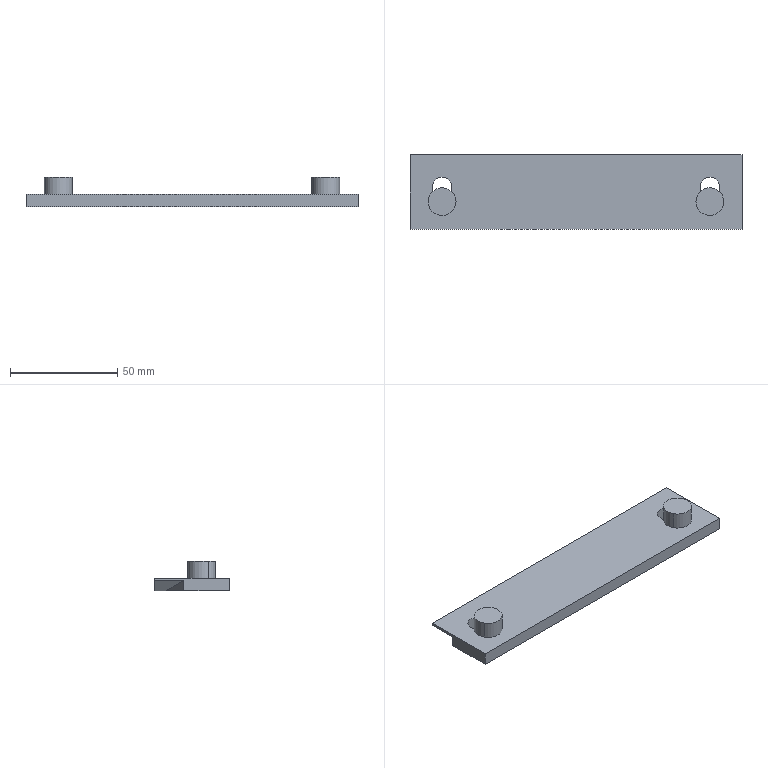Part | CATIA | 3 solids | 26 faces | box 155 x 35 x 14 mm | volume 32367 mm3 | plane 18 | cylinder 8 | commonest cylinder face diameters 9 x4 13 x4
STEP:
#1=CARTESIAN_POINT('',(-77.5,-30.,38.));
#2=VERTEX_POINT('',#1);
#3=CARTESIAN_POINT('',(-77.5,-30.,44.));
#4=VERTEX_POINT('',#3);
#5=CARTESIAN_POINT('',(-77.5,-30.,41.));
#6=DIRECTION('',(0.,0.,1.));
#7=VECTOR('',#6,1.);
#8=LINE('',#5,#7);
#9=EDGE_CURVE('',#2,#4,#8,.T.);
#10=ORIENTED_EDGE('',*,*,#9,.F.);
#11=CARTESIAN_POINT('',(77.5,-30.,38.));
#12=VERTEX_POINT('',#11);
#13=CARTESIAN_POINT('',(0.,-30.,38.));
#14=DIRECTION('',(1.,0.,0.));
#15=VECTOR('',#14,1.);
#16=LINE('',#13,#15);
#17=EDGE_CURVE('',#2,#12,#16,.T.);
#18=ORIENTED_EDGE('',*,*,#17,.T.);
#19=CARTESIAN_POINT('',(77.5,-30.,44.));
#20=VERTEX_POINT('',#19);
#21=CARTESIAN_POINT('',(77.5,-30.,41.));
#22=DIRECTION('',(0.,0.,1.));
#23=VECTOR('',#22,1.);
#24=LINE('',#21,#23);
#25=EDGE_CURVE('',#12,#20,#24,.T.);
#26=ORIENTED_EDGE('',*,*,#25,.T.);
#27=CARTESIAN_POINT('',(0.,-30.,44.));
#28=DIRECTION('',(1.,0.,0.));
#29=VECTOR('',#28,1.);
#30=LINE('',#27,#29);
#31=EDGE_CURVE('',#4,#20,#30,.T.);
#32=ORIENTED_EDGE('',*,*,#31,.F.);
#33=EDGE_LOOP('',(#10,#18,#26,#32));
#34=FACE_OUTER_BOUND('',#33,.T.);
#35=CARTESIAN_POINT('',(-77.5,-30.,38.));
#36=DIRECTION('',(0.,-1.,0.));
#37=DIRECTION('',(1.,0.,0.));
#38=AXIS2_PLACEMENT_3D('',#35,#36,#37);
#39=PLANE('',#38);
#40=ADVANCED_FACE('',(#34),#39,.T.);
#41=CARTESIAN_POINT('',(77.5,-8.66,42.874));
#42=VERTEX_POINT('',#41);
#43=CARTESIAN_POINT('',(77.5,-8.66,38.));
#44=VERTEX_POINT('',#43);
#45=CARTESIAN_POINT('',(77.5,-8.66,40.437));
#46=DIRECTION('',(0.,0.,-1.));
#47=VECTOR('',#46,1.);
#48=LINE('',#45,#47);
#49=EDGE_CURVE('',#42,#44,#48,.T.);
#50=ORIENTED_EDGE('',*,*,#49,.F.);
#51=CARTESIAN_POINT('',(77.5,5.,42.874));
#52=VERTEX_POINT('',#51);
#53=CARTESIAN_POINT('',(77.5,-1.83,42.874));
#54=DIRECTION('',(0.,1.,0.));
#55=VECTOR('',#54,1.);
#56=LINE('',#53,#55);
#57=EDGE_CURVE('',#42,#52,#56,.T.);
#58=ORIENTED_EDGE('',*,*,#57,.T.);
#59=CARTESIAN_POINT('',(77.5,5.,44.));
#60=VERTEX_POINT('',#59);
#61=CARTESIAN_POINT('',(77.5,5.,43.437));
#62=DIRECTION('',(0.,0.,1.));
#63=VECTOR('',#62,1.);
#64=LINE('',#61,#63);
#65=EDGE_CURVE('',#52,#60,#64,.T.);
#66=ORIENTED_EDGE('',*,*,#65,.T.);
#67=CARTESIAN_POINT('',(77.5,-12.5,44.));
#68=DIRECTION('',(0.,-1.,0.));
#69=VECTOR('',#68,1.);
#70=LINE('',#67,#69);
#71=EDGE_CURVE('',#20,#60,#70,.F.);
#72=ORIENTED_EDGE('',*,*,#71,.F.);
#73=ORIENTED_EDGE('',*,*,#25,.F.);
#74=CARTESIAN_POINT('',(77.5,-19.33,38.));
#75=DIRECTION('',(0.,-1.,0.));
#76=VECTOR('',#75,1.);
#77=LINE('',#74,#76);
#78=EDGE_CURVE('',#12,#44,#77,.F.);
#79=ORIENTED_EDGE('',*,*,#78,.T.);
#80=EDGE_LOOP('',(#50,#58,#66,#72,#73,#79));
#81=FACE_OUTER_BOUND('',#80,.T.);
#82=CARTESIAN_POINT('',(77.5,5.,38.));
#83=DIRECTION('',(-1.,0.,0.));
#84=DIRECTION('',(0.,-1.,0.));
#85=AXIS2_PLACEMENT_3D('',#82,#83,#84);
#86=PLANE('',#85);
#87=ADVANCED_FACE('',(#81),#86,.F.);
#88=CARTESIAN_POINT('',(-77.5,-8.66,42.874));
#89=VERTEX_POINT('',#88);
#90=CARTESIAN_POINT('',(-77.5,5.,42.874));
#91=VERTEX_POINT('',#90);
#92=CARTESIAN_POINT('',(-77.5,-1.83,42.874));
#93=DIRECTION('',(0.,1.,0.));
#94=VECTOR('',#93,1.);
#95=LINE('',#92,#94);
#96=EDGE_CURVE('',#89,#91,#95,.T.);
#97=ORIENTED_EDGE('',*,*,#96,.F.);
#98=CARTESIAN_POINT('',(-77.5,-8.66,38.));
#99=VERTEX_POINT('',#98);
#100=CARTESIAN_POINT('',(-77.5,-8.66,40.437));
#101=DIRECTION('',(0.,0.,-1.));
#102=VECTOR('',#101,1.);
#103=LINE('',#100,#102);
#104=EDGE_CURVE('',#89,#99,#103,.T.);
#105=ORIENTED_EDGE('',*,*,#104,.T.);
#106=CARTESIAN_POINT('',(-77.5,-19.33,38.));
#107=DIRECTION('',(0.,1.,0.));
#108=VECTOR('',#107,1.);
#109=LINE('',#106,#108);
#110=EDGE_CURVE('',#99,#2,#109,.F.);
#111=ORIENTED_EDGE('',*,*,#110,.T.);
#112=ORIENTED_EDGE('',*,*,#9,.T.);
#113=CARTESIAN_POINT('',(-77.5,5.,44.));
#114=VERTEX_POINT('',#113);
#115=CARTESIAN_POINT('',(-77.5,-12.5,44.));
#116=DIRECTION('',(0.,1.,0.));
#117=VECTOR('',#116,1.);
#118=LINE('',#115,#117);
#119=EDGE_CURVE('',#114,#4,#118,.F.);
#120=ORIENTED_EDGE('',*,*,#119,.F.);
#121=CARTESIAN_POINT('',(-77.5,5.,43.437));
#122=DIRECTION('',(0.,0.,1.));
#123=VECTOR('',#122,1.);
#124=LINE('',#121,#123);
#125=EDGE_CURVE('',#91,#114,#124,.T.);
#126=ORIENTED_EDGE('',*,*,#125,.F.);
#127=EDGE_LOOP('',(#97,#105,#111,#112,#120,#126));
#128=FACE_OUTER_BOUND('',#127,.T.);
#129=CARTESIAN_POINT('',(-77.5,-30.,38.));
#130=DIRECTION('',(1.,0.,0.));
#131=DIRECTION('',(0.,1.,0.));
#132=AXIS2_PLACEMENT_3D('',#129,#130,#131);
#133=PLANE('',#132);
#134=ADVANCED_FACE('',(#128),#133,.F.);
#135=CARTESIAN_POINT('',(62.5,5.,38.));
#136=VERTEX_POINT('',#135);
#137=CARTESIAN_POINT('',(-62.5,5.,38.));
#138=VERTEX_POINT('',#137);
#139=CARTESIAN_POINT('',(0.,5.,38.));
#140=DIRECTION('',(-1.,0.,0.));
#141=VECTOR('',#140,1.);
#142=LINE('',#139,#141);
#143=EDGE_CURVE('',#136,#138,#142,.T.);
#144=ORIENTED_EDGE('',*,*,#143,.T.);
#145=CARTESIAN_POINT('',(-70.,5.,40.437));
#146=DIRECTION('',(-0.9511,0.,0.309));
#147=VECTOR('',#146,1.);
#148=LINE('',#145,#147);
#149=EDGE_CURVE('',#138,#91,#148,.T.);
#150=ORIENTED_EDGE('',*,*,#149,.T.);
#151=ORIENTED_EDGE('',*,*,#125,.T.);
#152=CARTESIAN_POINT('',(0.,5.,44.));
#153=DIRECTION('',(-1.,0.,0.));
#154=VECTOR('',#153,1.);
#155=LINE('',#152,#154);
#156=EDGE_CURVE('',#60,#114,#155,.T.);
#157=ORIENTED_EDGE('',*,*,#156,.F.);
#158=ORIENTED_EDGE('',*,*,#65,.F.);
#159=CARTESIAN_POINT('',(70.,5.,40.437));
#160=DIRECTION('',(0.9511,0.,0.309));
#161=VECTOR('',#160,1.);
#162=LINE('',#159,#161);
#163=EDGE_CURVE('',#136,#52,#162,.T.);
#164=ORIENTED_EDGE('',*,*,#163,.F.);
#165=EDGE_LOOP('',(#144,#150,#151,#157,#158,#164));
#166=FACE_OUTER_BOUND('',#165,.T.);
#167=CARTESIAN_POINT('',(77.5,5.,38.));
#168=DIRECTION('',(0.,1.,0.));
#169=DIRECTION('',(-1.,0.,0.));
#170=AXIS2_PLACEMENT_3D('',#167,#168,#169);
#171=PLANE('',#170);
#172=ADVANCED_FACE('',(#166),#171,.T.);
#173=CARTESIAN_POINT('',(62.5,0.,38.));
#174=VERTEX_POINT('',#173);
#175=CARTESIAN_POINT('',(77.5,-8.66,42.874));
#176=CARTESIAN_POINT('',(62.5,0.,38.));
#177=B_SPLINE_CURVE_WITH_KNOTS('',1,(#175,#176),.UNSPECIFIED.,.F.,.U.,(2,2),(-2.999,14.994),.UNSPECIFIED.);
#178=EDGE_CURVE('',#174,#42,#177,.F.);
#179=ORIENTED_EDGE('',*,*,#178,.T.);
#180=ORIENTED_EDGE('',*,*,#49,.T.);
#181=CARTESIAN_POINT('',(75.,-7.217,38.));
#182=DIRECTION('',(0.866,-0.5,0.));
#183=VECTOR('',#182,1.);
#184=LINE('',#181,#183);
#185=EDGE_CURVE('',#174,#44,#184,.T.);
#186=ORIENTED_EDGE('',*,*,#185,.F.);
#187=EDGE_LOOP('',(#179,#180,#186));
#188=FACE_OUTER_BOUND('',#187,.T.);
#189=CARTESIAN_POINT('',(62.5,0.,38.));
#190=DIRECTION('',(0.5,0.866,0.));
#191=DIRECTION('',(0.,0.,1.));
#192=AXIS2_PLACEMENT_3D('',#189,#190,#191);
#193=PLANE('',#192);
#194=ADVANCED_FACE('',(#188),#193,.T.);
#195=ORIENTED_EDGE('',*,*,#163,.T.);
#196=ORIENTED_EDGE('',*,*,#57,.F.);
#197=ORIENTED_EDGE('',*,*,#178,.F.);
#198=CARTESIAN_POINT('',(62.5,5.,38.));
#199=DIRECTION('',(0.,-1.,0.));
#200=VECTOR('',#199,1.);
#201=LINE('',#198,#200);
#202=EDGE_CURVE('',#174,#136,#201,.F.);
#203=ORIENTED_EDGE('',*,*,#202,.T.);
#204=EDGE_LOOP('',(#195,#196,#197,#203));
#205=FACE_OUTER_BOUND('',#204,.T.);
#206=CARTESIAN_POINT('',(62.5,10.,38.));
#207=DIRECTION('',(-0.309,0.,0.9511));
#208=DIRECTION('',(0.,-1.,0.));
#209=AXIS2_PLACEMENT_3D('',#206,#207,#208);
#210=PLANE('',#209);
#211=ADVANCED_FACE('',(#205),#210,.F.);
#212=CARTESIAN_POINT('',(-62.5,0.,38.));
#213=VERTEX_POINT('',#212);
#214=CARTESIAN_POINT('',(-75.,-7.217,38.));
#215=DIRECTION('',(-0.866,-0.5,0.));
#216=VECTOR('',#215,1.);
#217=LINE('',#214,#216);
#218=EDGE_CURVE('',#213,#99,#217,.T.);
#219=ORIENTED_EDGE('',*,*,#218,.T.);
#220=ORIENTED_EDGE('',*,*,#104,.F.);
#221=CARTESIAN_POINT('',(-77.5,-8.66,42.874));
#222=CARTESIAN_POINT('',(-62.5,0.,38.));
#223=B_SPLINE_CURVE_WITH_KNOTS('',1,(#221,#222),.UNSPECIFIED.,.F.,.U.,(2,2),(-2.999,14.994),.UNSPECIFIED.);
#224=EDGE_CURVE('',#213,#89,#223,.F.);
#225=ORIENTED_EDGE('',*,*,#224,.F.);
#226=EDGE_LOOP('',(#219,#220,#225));
#227=FACE_OUTER_BOUND('',#226,.T.);
#228=CARTESIAN_POINT('',(-62.5,0.,38.));
#229=DIRECTION('',(0.5,-0.866,0.));
#230=DIRECTION('',(0.,0.,1.));
#231=AXIS2_PLACEMENT_3D('',#228,#229,#230);
#232=PLANE('',#231);
#233=ADVANCED_FACE('',(#227),#232,.F.);
#234=CARTESIAN_POINT('',(-62.5,5.,38.));
#235=DIRECTION('',(0.,-1.,0.));
#236=VECTOR('',#235,1.);
#237=LINE('',#234,#236);
#238=EDGE_CURVE('',#213,#138,#237,.F.);
#239=ORIENTED_EDGE('',*,*,#238,.F.);
#240=ORIENTED_EDGE('',*,*,#224,.T.);
#241=ORIENTED_EDGE('',*,*,#96,.T.);
#242=ORIENTED_EDGE('',*,*,#149,.F.);
#243=EDGE_LOOP('',(#239,#240,#241,#242));
#244=FACE_OUTER_BOUND('',#243,.T.);
#245=CARTESIAN_POINT('',(-62.5,10.,38.));
#246=DIRECTION('',(-0.309,0.,-0.9511));
#247=DIRECTION('',(0.,-1.,0.));
#248=AXIS2_PLACEMENT_3D('',#245,#246,#247);
#249=PLANE('',#248);
#250=ADVANCED_FACE('',(#244),#249,.T.);
#251=ORIENTED_EDGE('',*,*,#143,.F.);
#252=ORIENTED_EDGE('',*,*,#202,.F.);
#253=ORIENTED_EDGE('',*,*,#185,.T.);
#254=ORIENTED_EDGE('',*,*,#78,.F.);
#255=ORIENTED_EDGE('',*,*,#17,.F.);
#256=ORIENTED_EDGE('',*,*,#110,.F.);
#257=ORIENTED_EDGE('',*,*,#218,.F.);
#258=ORIENTED_EDGE('',*,*,#238,.T.);
#259=EDGE_LOOP('',(#251,#252,#253,#254,#255,#256,#257,#258));
#260=FACE_OUTER_BOUND('',#259,.T.);
#261=CARTESIAN_POINT('',(-58.,-10.,38.));
#262=VERTEX_POINT('',#261);
#263=CARTESIAN_POINT('',(-58.,-17.,38.));
#264=VERTEX_POINT('',#263);
#265=CARTESIAN_POINT('',(-58.,-13.5,38.));
#266=DIRECTION('',(0.,-1.,0.));
#267=VECTOR('',#266,1.);
#268=LINE('',#265,#267);
#269=EDGE_CURVE('',#262,#264,#268,.T.);
#270=ORIENTED_EDGE('',*,*,#269,.F.);
#271=CARTESIAN_POINT('',(-67.,-10.,38.));
#272=VERTEX_POINT('',#271);
#273=CARTESIAN_POINT('',(-62.5,-10.,38.));
#274=DIRECTION('',(0.,0.,1.));
#275=AXIS2_PLACEMENT_3D('',#273,#274,$);
#276=CIRCLE('',#275,4.5);
#277=EDGE_CURVE('',#262,#272,#276,.T.);
#278=ORIENTED_EDGE('',*,*,#277,.T.);
#279=CARTESIAN_POINT('',(-67.,-17.,38.));
#280=VERTEX_POINT('',#279);
#281=CARTESIAN_POINT('',(-67.,-13.5,38.));
#282=DIRECTION('',(0.,-1.,0.));
#283=VECTOR('',#282,1.);
#284=LINE('',#281,#283);
#285=EDGE_CURVE('',#272,#280,#284,.T.);
#286=ORIENTED_EDGE('',*,*,#285,.T.);
#287=CARTESIAN_POINT('',(-62.5,-17.,38.));
#288=DIRECTION('',(0.,0.,1.));
#289=AXIS2_PLACEMENT_3D('',#287,#288,$);
#290=CIRCLE('',#289,4.5);
#291=EDGE_CURVE('',#280,#264,#290,.T.);
#292=ORIENTED_EDGE('',*,*,#291,.T.);
#293=EDGE_LOOP('',(#270,#278,#286,#292));
#294=FACE_BOUND('',#293,.T.);
#295=CARTESIAN_POINT('',(67.,-10.,38.));
#296=VERTEX_POINT('',#295);
#297=CARTESIAN_POINT('',(58.,-10.,38.));
#298=VERTEX_POINT('',#297);
#299=CARTESIAN_POINT('',(62.5,-10.,38.));
#300=DIRECTION('',(0.,0.,1.));
#301=AXIS2_PLACEMENT_3D('',#299,#300,$);
#302=CIRCLE('',#301,4.5);
#303=EDGE_CURVE('',#296,#298,#302,.T.);
#304=ORIENTED_EDGE('',*,*,#303,.T.);
#305=CARTESIAN_POINT('',(58.,-17.,38.));
#306=VERTEX_POINT('',#305);
#307=CARTESIAN_POINT('',(58.,-13.5,38.));
#308=DIRECTION('',(0.,-1.,0.));
#309=VECTOR('',#308,1.);
#310=LINE('',#307,#309);
#311=EDGE_CURVE('',#298,#306,#310,.T.);
#312=ORIENTED_EDGE('',*,*,#311,.T.);
#313=CARTESIAN_POINT('',(67.,-17.,38.));
#314=VERTEX_POINT('',#313);
#315=CARTESIAN_POINT('',(62.5,-17.,38.));
#316=DIRECTION('',(0.,0.,1.));
#317=AXIS2_PLACEMENT_3D('',#315,#316,$);
#318=CIRCLE('',#317,4.5);
#319=EDGE_CURVE('',#306,#314,#318,.T.);
#320=ORIENTED_EDGE('',*,*,#319,.T.);
#321=CARTESIAN_POINT('',(67.,-13.5,38.));
#322=DIRECTION('',(0.,-1.,0.));
#323=VECTOR('',#322,1.);
#324=LINE('',#321,#323);
#325=EDGE_CURVE('',#296,#314,#324,.T.);
#326=ORIENTED_EDGE('',*,*,#325,.F.);
#327=EDGE_LOOP('',(#304,#312,#320,#326));
#328=FACE_BOUND('',#327,.T.);
#329=CARTESIAN_POINT('',(0.,0.,38.));
#330=DIRECTION('',(0.,0.,1.));
#331=DIRECTION('',(1.,0.,0.));
#332=AXIS2_PLACEMENT_3D('',#329,#330,#331);
#333=PLANE('',#332);
#334=ADVANCED_FACE('',(#260,#294,#328),#333,.F.);
#335=ORIENTED_EDGE('',*,*,#156,.T.);
#336=ORIENTED_EDGE('',*,*,#119,.T.);
#337=ORIENTED_EDGE('',*,*,#31,.T.);
#338=ORIENTED_EDGE('',*,*,#71,.T.);
#339=EDGE_LOOP('',(#335,#336,#337,#338));
#340=FACE_OUTER_BOUND('',#339,.T.);
#341=CARTESIAN_POINT('',(-58.,-17.,44.));
#342=VERTEX_POINT('',#341);
#343=CARTESIAN_POINT('',(-58.,-10.,44.));
#344=VERTEX_POINT('',#343);
#345=CARTESIAN_POINT('',(-58.,-13.5,44.));
#346=DIRECTION('',(0.,-1.,0.));
#347=VECTOR('',#346,1.);
#348=LINE('',#345,#347);
#349=EDGE_CURVE('',#342,#344,#348,.F.);
#350=ORIENTED_EDGE('',*,*,#349,.F.);
#351=CARTESIAN_POINT('',(-67.,-17.,44.));
#352=VERTEX_POINT('',#351);
#353=CARTESIAN_POINT('',(-62.5,-17.,44.));
#354=DIRECTION('',(0.,0.,1.));
#355=AXIS2_PLACEMENT_3D('',#353,#354,$);
#356=CIRCLE('',#355,4.5);
#357=EDGE_CURVE('',#352,#342,#356,.T.);
#358=ORIENTED_EDGE('',*,*,#357,.F.);
#359=CARTESIAN_POINT('',(-67.,-10.,44.));
#360=VERTEX_POINT('',#359);
#361=CARTESIAN_POINT('',(-67.,-13.5,44.));
#362=DIRECTION('',(0.,-1.,0.));
#363=VECTOR('',#362,1.);
#364=LINE('',#361,#363);
#365=EDGE_CURVE('',#360,#352,#364,.T.);
#366=ORIENTED_EDGE('',*,*,#365,.F.);
#367=CARTESIAN_POINT('',(-62.5,-10.,44.));
#368=DIRECTION('',(0.,0.,1.));
#369=AXIS2_PLACEMENT_3D('',#367,#368,$);
#370=CIRCLE('',#369,4.5);
#371=EDGE_CURVE('',#344,#360,#370,.T.);
#372=ORIENTED_EDGE('',*,*,#371,.F.);
#373=EDGE_LOOP('',(#350,#358,#366,#372));
#374=FACE_BOUND('',#373,.T.);
#375=CARTESIAN_POINT('',(67.,-10.,44.));
#376=VERTEX_POINT('',#375);
#377=CARTESIAN_POINT('',(58.,-10.,44.));
#378=VERTEX_POINT('',#377);
#379=CARTESIAN_POINT('',(62.5,-10.,44.));
#380=DIRECTION('',(0.,0.,1.));
#381=AXIS2_PLACEMENT_3D('',#379,#380,$);
#382=CIRCLE('',#381,4.5);
#383=EDGE_CURVE('',#376,#378,#382,.T.);
#384=ORIENTED_EDGE('',*,*,#383,.F.);
#385=CARTESIAN_POINT('',(67.,-17.,44.));
#386=VERTEX_POINT('',#385);
#387=CARTESIAN_POINT('',(67.,-13.5,44.));
#388=DIRECTION('',(0.,-1.,0.));
#389=VECTOR('',#388,1.);
#390=LINE('',#387,#389);
#391=EDGE_CURVE('',#386,#376,#390,.F.);
#392=ORIENTED_EDGE('',*,*,#391,.F.);
#393=CARTESIAN_POINT('',(58.,-17.,44.));
#394=VERTEX_POINT('',#393);
#395=CARTESIAN_POINT('',(62.5,-17.,44.));
#396=DIRECTION('',(0.,0.,1.));
#397=AXIS2_PLACEMENT_3D('',#395,#396,$);
#398=CIRCLE('',#397,4.5);
#399=EDGE_CURVE('',#394,#386,#398,.T.);
#400=ORIENTED_EDGE('',*,*,#399,.F.);
#401=CARTESIAN_POINT('',(58.,-13.5,44.));
#402=DIRECTION('',(0.,-1.,0.));
#403=VECTOR('',#402,1.);
#404=LINE('',#401,#403);
#405=EDGE_CURVE('',#378,#394,#404,.T.);
#406=ORIENTED_EDGE('',*,*,#405,.F.);
#407=EDGE_LOOP('',(#384,#392,#400,#406));
#408=FACE_BOUND('',#407,.T.);
#409=CARTESIAN_POINT('',(0.,0.,44.));
#410=DIRECTION('',(0.,0.,1.));
#411=DIRECTION('',(1.,0.,0.));
#412=AXIS2_PLACEMENT_3D('',#409,#410,#411);
#413=PLANE('',#412);
#414=ADVANCED_FACE('',(#340,#374,#408),#413,.T.);
#415=ORIENTED_EDGE('',*,*,#303,.F.);
#416=CARTESIAN_POINT('',(67.,-10.,34.));
#417=DIRECTION('',(0.,0.,1.));
#418=VECTOR('',#417,1.);
#419=LINE('',#416,#418);
#420=EDGE_CURVE('',#376,#296,#419,.F.);
#421=ORIENTED_EDGE('',*,*,#420,.F.);
#422=ORIENTED_EDGE('',*,*,#383,.T.);
#423=CARTESIAN_POINT('',(58.,-10.,34.));
#424=DIRECTION('',(0.,0.,1.));
#425=VECTOR('',#424,1.);
#426=LINE('',#423,#425);
#427=EDGE_CURVE('',#378,#298,#426,.F.);
#428=ORIENTED_EDGE('',*,*,#427,.T.);
#429=EDGE_LOOP('',(#415,#421,#422,#428));
#430=FACE_OUTER_BOUND('',#429,.T.);
#431=CARTESIAN_POINT('',(62.5,-10.,34.));
#432=DIRECTION('',(0.,0.,1.));
#433=DIRECTION('',(1.,0.,0.));
#434=AXIS2_PLACEMENT_3D('',#431,#432,#433);
#435=CYLINDRICAL_SURFACE('',#434,4.5);
#436=ADVANCED_FACE('',(#430),#435,.F.);
#437=ORIENTED_EDGE('',*,*,#427,.F.);
#438=ORIENTED_EDGE('',*,*,#405,.T.);
#439=CARTESIAN_POINT('',(58.,-17.,41.));
#440=DIRECTION('',(0.,0.,-1.));
#441=VECTOR('',#440,1.);
#442=LINE('',#439,#441);
#443=EDGE_CURVE('',#394,#306,#442,.T.);
#444=ORIENTED_EDGE('',*,*,#443,.T.);
#445=ORIENTED_EDGE('',*,*,#311,.F.);
#446=EDGE_LOOP('',(#437,#438,#444,#445));
#447=FACE_OUTER_BOUND('',#446,.T.);
#448=CARTESIAN_POINT('',(58.,-10.,44.));
#449=DIRECTION('',(1.,0.,0.));
#450=DIRECTION('',(0.,-1.,0.));
#451=AXIS2_PLACEMENT_3D('',#448,#449,#450);
#452=PLANE('',#451);
#453=ADVANCED_FACE('',(#447),#452,.T.);
#454=ORIENTED_EDGE('',*,*,#325,.T.);
#455=CARTESIAN_POINT('',(67.,-17.,41.));
#456=DIRECTION('',(0.,0.,-1.));
#457=VECTOR('',#456,1.);
#458=LINE('',#455,#457);
#459=EDGE_CURVE('',#386,#314,#458,.T.);
#460=ORIENTED_EDGE('',*,*,#459,.F.);
#461=ORIENTED_EDGE('',*,*,#391,.T.);
#462=ORIENTED_EDGE('',*,*,#420,.T.);
#463=EDGE_LOOP('',(#454,#460,#461,#462));
#464=FACE_OUTER_BOUND('',#463,.T.);
#465=CARTESIAN_POINT('',(67.,-10.,44.));
#466=DIRECTION('',(1.,0.,0.));
#467=DIRECTION('',(0.,-1.,0.));
#468=AXIS2_PLACEMENT_3D('',#465,#466,#467);
#469=PLANE('',#468);
#470=ADVANCED_FACE('',(#464),#469,.F.);
#471=ORIENTED_EDGE('',*,*,#319,.F.);
#472=ORIENTED_EDGE('',*,*,#443,.F.);
#473=ORIENTED_EDGE('',*,*,#399,.T.);
#474=ORIENTED_EDGE('',*,*,#459,.T.);
#475=EDGE_LOOP('',(#471,#472,#473,#474));
#476=FACE_OUTER_BOUND('',#475,.T.);
#477=CARTESIAN_POINT('',(62.5,-17.,34.));
#478=DIRECTION('',(0.,0.,1.));
#479=DIRECTION('',(-1.,0.,0.));
#480=AXIS2_PLACEMENT_3D('',#477,#478,#479);
#481=CYLINDRICAL_SURFACE('',#480,4.5);
#482=ADVANCED_FACE('',(#476),#481,.F.);
#483=ORIENTED_EDGE('',*,*,#269,.T.);
#484=CARTESIAN_POINT('',(-58.,-17.,41.));
#485=DIRECTION('',(0.,0.,-1.));
#486=VECTOR('',#485,1.);
#487=LINE('',#484,#486);
#488=EDGE_CURVE('',#342,#264,#487,.T.);
#489=ORIENTED_EDGE('',*,*,#488,.F.);
#490=ORIENTED_EDGE('',*,*,#349,.T.);
#491=CARTESIAN_POINT('',(-58.,-10.,41.));
#492=DIRECTION('',(0.,0.,-1.));
#493=VECTOR('',#492,1.);
#494=LINE('',#491,#493);
#495=EDGE_CURVE('',#344,#262,#494,.T.);
#496=ORIENTED_EDGE('',*,*,#495,.T.);
#497=EDGE_LOOP('',(#483,#489,#490,#496));
#498=FACE_OUTER_BOUND('',#497,.T.);
#499=CARTESIAN_POINT('',(-58.,-10.,44.));
#500=DIRECTION('',(1.,0.,0.));
#501=DIRECTION('',(0.,-1.,0.));
#502=AXIS2_PLACEMENT_3D('',#499,#500,#501);
#503=PLANE('',#502);
#504=ADVANCED_FACE('',(#498),#503,.F.);
#505=ORIENTED_EDGE('',*,*,#277,.F.);
#506=ORIENTED_EDGE('',*,*,#495,.F.);
#507=ORIENTED_EDGE('',*,*,#371,.T.);
#508=CARTESIAN_POINT('',(-67.,-10.,34.));
#509=DIRECTION('',(0.,0.,1.));
#510=VECTOR('',#509,1.);
#511=LINE('',#508,#510);
#512=EDGE_CURVE('',#360,#272,#511,.F.);
#513=ORIENTED_EDGE('',*,*,#512,.T.);
#514=EDGE_LOOP('',(#505,#506,#507,#513));
#515=FACE_OUTER_BOUND('',#514,.T.);
#516=CARTESIAN_POINT('',(-62.5,-10.,34.));
#517=DIRECTION('',(0.,0.,1.));
#518=DIRECTION('',(1.,0.,0.));
#519=AXIS2_PLACEMENT_3D('',#516,#517,#518);
#520=CYLINDRICAL_SURFACE('',#519,4.5);
#521=ADVANCED_FACE('',(#515),#520,.F.);
#522=ORIENTED_EDGE('',*,*,#291,.F.);
#523=CARTESIAN_POINT('',(-67.,-17.,34.));
#524=DIRECTION('',(0.,0.,1.));
#525=VECTOR('',#524,1.);
#526=LINE('',#523,#525);
#527=EDGE_CURVE('',#352,#280,#526,.F.);
#528=ORIENTED_EDGE('',*,*,#527,.F.);
#529=ORIENTED_EDGE('',*,*,#357,.T.);
#530=ORIENTED_EDGE('',*,*,#488,.T.);
#531=EDGE_LOOP('',(#522,#528,#529,#530));
#532=FACE_OUTER_BOUND('',#531,.T.);
#533=CARTESIAN_POINT('',(-62.5,-17.,34.));
#534=DIRECTION('',(0.,0.,1.));
#535=DIRECTION('',(-1.,0.,0.));
#536=AXIS2_PLACEMENT_3D('',#533,#534,#535);
#537=CYLINDRICAL_SURFACE('',#536,4.5);
#538=ADVANCED_FACE('',(#532),#537,.F.);
#539=ORIENTED_EDGE('',*,*,#512,.F.);
#540=ORIENTED_EDGE('',*,*,#365,.T.);
#541=ORIENTED_EDGE('',*,*,#527,.T.);
#542=ORIENTED_EDGE('',*,*,#285,.F.);
#543=EDGE_LOOP('',(#539,#540,#541,#542));
#544=FACE_OUTER_BOUND('',#543,.T.);
#545=CARTESIAN_POINT('',(-67.,-10.,44.));
#546=DIRECTION('',(1.,0.,0.));
#547=DIRECTION('',(0.,-1.,0.));
#548=AXIS2_PLACEMENT_3D('',#545,#546,#547);
#549=PLANE('',#548);
#550=ADVANCED_FACE('',(#544),#549,.T.);
#551=CLOSED_SHELL('',(#40,#87,#134,#172,#194,#211,#233,#250,#334,#414,#436,#453,#470,#482,#504,#521,#538,#550));
#552=MANIFOLD_SOLID_BREP('',#551);
#553=CARTESIAN_POINT('',(-56.796,-13.884,52.));
#554=VERTEX_POINT('',#553);
#555=CARTESIAN_POINT('',(-68.204,-20.116,52.));
#556=VERTEX_POINT('',#555);
#557=CARTESIAN_POINT('',(-62.5,-17.,52.));
#558=DIRECTION('',(0.,0.,1.));
#559=AXIS2_PLACEMENT_3D('',#557,#558,$);
#560=CIRCLE('',#559,6.5);
#561=EDGE_CURVE('',#554,#556,#560,.T.);
#562=ORIENTED_EDGE('',*,*,#561,.T.);
#563=CARTESIAN_POINT('',(-62.5,-17.,52.));
#564=DIRECTION('',(0.,0.,1.));
#565=AXIS2_PLACEMENT_3D('',#563,#564,$);
#566=CIRCLE('',#565,6.5);
#567=EDGE_CURVE('',#556,#554,#566,.T.);
#568=ORIENTED_EDGE('',*,*,#567,.T.);
#569=EDGE_LOOP('',(#562,#568));
#570=FACE_OUTER_BOUND('',#569,.T.);
#571=CARTESIAN_POINT('',(-62.5,-17.,52.));
#572=DIRECTION('',(0.,0.,1.));
#573=DIRECTION('',(1.,0.,0.));
#574=AXIS2_PLACEMENT_3D('',#571,#572,#573);
#575=PLANE('',#574);
#576=ADVANCED_FACE('',(#570),#575,.T.);
#577=CARTESIAN_POINT('',(-68.204,-20.116,44.));
#578=VERTEX_POINT('',#577);
#579=CARTESIAN_POINT('',(-68.204,-20.116,47.8));
#580=DIRECTION('',(0.,0.,1.));
#581=VECTOR('',#580,1.);
#582=LINE('',#579,#581);
#583=EDGE_CURVE('',#556,#578,#582,.F.);
#584=ORIENTED_EDGE('',*,*,#583,.F.);
#585=ORIENTED_EDGE('',*,*,#561,.F.);
#586=CARTESIAN_POINT('',(-56.796,-13.884,44.));
#587=VERTEX_POINT('',#586);
#588=CARTESIAN_POINT('',(-56.796,-13.884,47.8));
#589=DIRECTION('',(0.,0.,1.));
#590=VECTOR('',#589,1.);
#591=LINE('',#588,#590);
#592=EDGE_CURVE('',#554,#587,#591,.F.);
#593=ORIENTED_EDGE('',*,*,#592,.T.);
#594=CARTESIAN_POINT('',(-62.5,-17.,44.));
#595=DIRECTION('',(0.,0.,1.));
#596=AXIS2_PLACEMENT_3D('',#594,#595,$);
#597=CIRCLE('',#596,6.5);
#598=EDGE_CURVE('',#587,#578,#597,.T.);
#599=ORIENTED_EDGE('',*,*,#598,.T.);
#600=EDGE_LOOP('',(#584,#585,#593,#599));
#601=FACE_OUTER_BOUND('',#600,.T.);
#602=CARTESIAN_POINT('',(-62.5,-17.,44.1));
#603=DIRECTION('',(0.,0.,1.));
#604=DIRECTION('',(0.8776,0.4794,0.));
#605=AXIS2_PLACEMENT_3D('',#602,#603,#604);
#606=CYLINDRICAL_SURFACE('',#605,6.5);
#607=ADVANCED_FACE('',(#601),#606,.T.);
#608=ORIENTED_EDGE('',*,*,#592,.F.);
#609=ORIENTED_EDGE('',*,*,#567,.F.);
#610=ORIENTED_EDGE('',*,*,#583,.T.);
#611=CARTESIAN_POINT('',(-62.5,-17.,44.));
#612=DIRECTION('',(0.,0.,1.));
#613=AXIS2_PLACEMENT_3D('',#611,#612,$);
#614=CIRCLE('',#613,6.5);
#615=EDGE_CURVE('',#578,#587,#614,.T.);
#616=ORIENTED_EDGE('',*,*,#615,.T.);
#617=EDGE_LOOP('',(#608,#609,#610,#616));
#618=FACE_OUTER_BOUND('',#617,.T.);
#619=ADVANCED_FACE('',(#618),#606,.T.);
#620=ORIENTED_EDGE('',*,*,#598,.F.);
#621=ORIENTED_EDGE('',*,*,#615,.F.);
#622=EDGE_LOOP('',(#620,#621));
#623=FACE_OUTER_BOUND('',#622,.T.);
#624=ADVANCED_FACE('',(#623),#413,.F.);
#625=CLOSED_SHELL('',(#576,#607,#619,#624));
#626=MANIFOLD_SOLID_BREP('',#625);
#627=CARTESIAN_POINT('',(68.204,-13.884,52.));
#628=VERTEX_POINT('',#627);
#629=CARTESIAN_POINT('',(56.796,-20.116,52.));
#630=VERTEX_POINT('',#629);
#631=CARTESIAN_POINT('',(62.5,-17.,52.));
#632=DIRECTION('',(0.,0.,1.));
#633=AXIS2_PLACEMENT_3D('',#631,#632,$);
#634=CIRCLE('',#633,6.5);
#635=EDGE_CURVE('',#628,#630,#634,.T.);
#636=ORIENTED_EDGE('',*,*,#635,.T.);
#637=CARTESIAN_POINT('',(62.5,-17.,52.));
#638=DIRECTION('',(0.,0.,1.));
#639=AXIS2_PLACEMENT_3D('',#637,#638,$);
#640=CIRCLE('',#639,6.5);
#641=EDGE_CURVE('',#630,#628,#640,.T.);
#642=ORIENTED_EDGE('',*,*,#641,.T.);
#643=EDGE_LOOP('',(#636,#642));
#644=FACE_OUTER_BOUND('',#643,.T.);
#645=ADVANCED_FACE('',(#644),#575,.T.);
#646=CARTESIAN_POINT('',(56.796,-20.116,44.));
#647=VERTEX_POINT('',#646);
#648=CARTESIAN_POINT('',(56.796,-20.116,47.8));
#649=DIRECTION('',(0.,0.,1.));
#650=VECTOR('',#649,1.);
#651=LINE('',#648,#650);
#652=EDGE_CURVE('',#630,#647,#651,.F.);
#653=ORIENTED_EDGE('',*,*,#652,.F.);
#654=ORIENTED_EDGE('',*,*,#635,.F.);
#655=CARTESIAN_POINT('',(68.204,-13.884,44.));
#656=VERTEX_POINT('',#655);
#657=CARTESIAN_POINT('',(68.204,-13.884,47.8));
#658=DIRECTION('',(0.,0.,1.));
#659=VECTOR('',#658,1.);
#660=LINE('',#657,#659);
#661=EDGE_CURVE('',#628,#656,#660,.F.);
#662=ORIENTED_EDGE('',*,*,#661,.T.);
#663=CARTESIAN_POINT('',(62.5,-17.,44.));
#664=DIRECTION('',(0.,0.,1.));
#665=AXIS2_PLACEMENT_3D('',#663,#664,$);
#666=CIRCLE('',#665,6.5);
#667=EDGE_CURVE('',#656,#647,#666,.T.);
#668=ORIENTED_EDGE('',*,*,#667,.T.);
#669=EDGE_LOOP('',(#653,#654,#662,#668));
#670=FACE_OUTER_BOUND('',#669,.T.);
#671=CARTESIAN_POINT('',(62.5,-17.,44.1));
#672=DIRECTION('',(0.,0.,1.));
#673=DIRECTION('',(0.8776,0.4794,0.));
#674=AXIS2_PLACEMENT_3D('',#671,#672,#673);
#675=CYLINDRICAL_SURFACE('',#674,6.5);
#676=ADVANCED_FACE('',(#670),#675,.T.);
#677=ORIENTED_EDGE('',*,*,#661,.F.);
#678=ORIENTED_EDGE('',*,*,#641,.F.);
#679=ORIENTED_EDGE('',*,*,#652,.T.);
#680=CARTESIAN_POINT('',(62.5,-17.,44.));
#681=DIRECTION('',(0.,0.,1.));
#682=AXIS2_PLACEMENT_3D('',#680,#681,$);
#683=CIRCLE('',#682,6.5);
#684=EDGE_CURVE('',#647,#656,#683,.T.);
#685=ORIENTED_EDGE('',*,*,#684,.T.);
#686=EDGE_LOOP('',(#677,#678,#679,#685));
#687=FACE_OUTER_BOUND('',#686,.T.);
#688=ADVANCED_FACE('',(#687),#675,.T.);
#689=ORIENTED_EDGE('',*,*,#667,.F.);
#690=ORIENTED_EDGE('',*,*,#684,.F.);
#691=EDGE_LOOP('',(#689,#690));
#692=FACE_OUTER_BOUND('',#691,.T.);
#693=ADVANCED_FACE('',(#692),#413,.F.);
#694=CLOSED_SHELL('',(#645,#676,#688,#693));
#695=MANIFOLD_SOLID_BREP('',#694);
#696=(LENGTH_UNIT()NAMED_UNIT(*)SI_UNIT(.MILLI.,.METRE.));
#697=UNCERTAINTY_MEASURE_WITH_UNIT(LENGTH_MEASURE(0.005),#696,'','');
#698=(NAMED_UNIT(*)PLANE_ANGLE_UNIT()SI_UNIT($,.RADIAN.));
#699=(NAMED_UNIT(*)SI_UNIT($,.STERADIAN.)SOLID_ANGLE_UNIT());
#700=(GEOMETRIC_REPRESENTATION_CONTEXT(3)GLOBAL_UNCERTAINTY_ASSIGNED_CONTEXT((#697))GLOBAL_UNIT_ASSIGNED_CONTEXT((#696,#698,#699))REPRESENTATION_CONTEXT('',''));
#701=ADVANCED_BREP_SHAPE_REPRESENTATION('',(#552,#626,#695),#700);